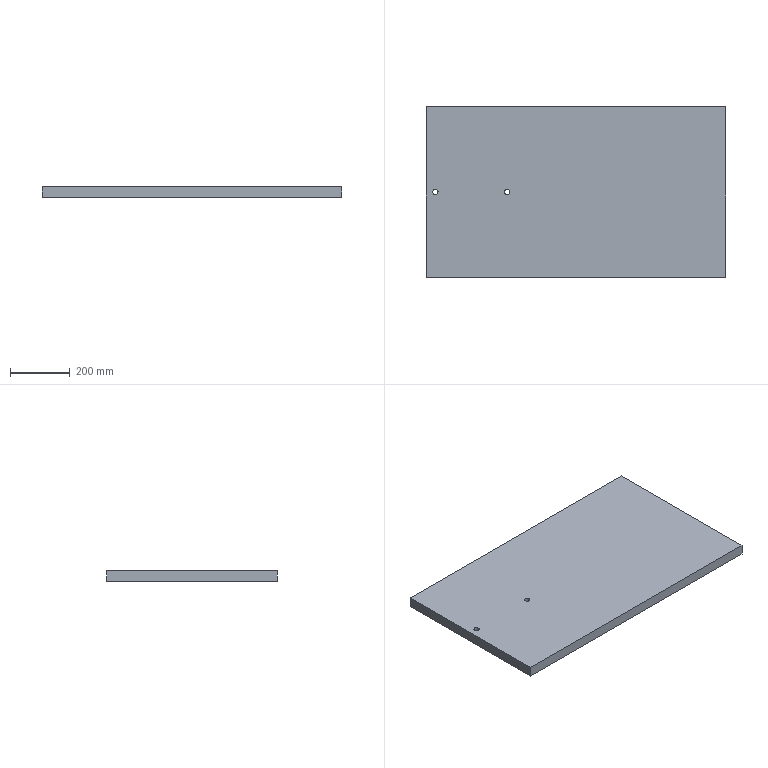Part | SolidWorks | features 3DProfileFeature 1, Extrusion 1, HoleWzd 1 | 1 solid | 10 faces | box 1000 x 570 x 35 mm | volume 19933163 mm3 | plane 6 | cylinder 4 | commonest cylinder face diameters 17.5 x4
STEP:
#1=CARTESIAN_POINT('',(21.25,285.,0.));
#2=VERTEX_POINT('',#1);
#3=CARTESIAN_POINT('',(38.75,285.,0.));
#4=VERTEX_POINT('',#3);
#5=CARTESIAN_POINT('',(30.,285.,0.));
#6=DIRECTION('',(0.,0.,1.));
#7=DIRECTION('',(1.,0.,0.));
#8=AXIS2_PLACEMENT_3D('',#5,#6,#7);
#9=CIRCLE('',#8,8.75);
#10=EDGE_CURVE('',#2,#4,#9,.T.);
#11=ORIENTED_EDGE('',*,*,#10,.F.);
#12=CARTESIAN_POINT('',(21.25,285.,35.));
#13=VERTEX_POINT('',#12);
#14=CARTESIAN_POINT('',(21.25,285.,35.));
#15=DIRECTION('',(0.,0.,1.));
#16=VECTOR('',#15,1000.);
#17=LINE('',#14,#16);
#18=EDGE_CURVE('',#2,#13,#17,.T.);
#19=ORIENTED_EDGE('',*,*,#18,.T.);
#20=CARTESIAN_POINT('',(38.75,285.,35.));
#21=VERTEX_POINT('',#20);
#22=CARTESIAN_POINT('',(30.,285.,35.));
#23=DIRECTION('',(0.,0.,1.));
#24=DIRECTION('',(1.,0.,0.));
#25=AXIS2_PLACEMENT_3D('',#22,#23,#24);
#26=CIRCLE('',#25,8.75);
#27=EDGE_CURVE('',#13,#21,#26,.T.);
#28=ORIENTED_EDGE('',*,*,#27,.T.);
#29=CARTESIAN_POINT('',(38.75,285.,35.));
#30=DIRECTION('',(0.,0.,1.));
#31=VECTOR('',#30,1000.);
#32=LINE('',#29,#31);
#33=EDGE_CURVE('',#4,#21,#32,.T.);
#34=ORIENTED_EDGE('',*,*,#33,.F.);
#35=EDGE_LOOP('',(#11,#19,#28,#34));
#36=FACE_OUTER_BOUND('',#35,.T.);
#37=CARTESIAN_POINT('',(30.,285.,35.));
#38=DIRECTION('',(0.,0.,1.));
#39=DIRECTION('',(1.,0.,0.));
#40=AXIS2_PLACEMENT_3D('',#37,#38,#39);
#41=CYLINDRICAL_SURFACE('',#40,8.75);
#42=ADVANCED_FACE('',(#36),#41,.F.);
#43=CARTESIAN_POINT('',(261.25,285.,0.));
#44=VERTEX_POINT('',#43);
#45=CARTESIAN_POINT('',(278.75,285.,0.));
#46=VERTEX_POINT('',#45);
#47=CARTESIAN_POINT('',(270.,285.,0.));
#48=DIRECTION('',(0.,0.,1.));
#49=DIRECTION('',(1.,0.,0.));
#50=AXIS2_PLACEMENT_3D('',#47,#48,#49);
#51=CIRCLE('',#50,8.75);
#52=EDGE_CURVE('',#44,#46,#51,.T.);
#53=ORIENTED_EDGE('',*,*,#52,.F.);
#54=CARTESIAN_POINT('',(261.25,285.,35.));
#55=VERTEX_POINT('',#54);
#56=CARTESIAN_POINT('',(261.25,285.,35.));
#57=DIRECTION('',(0.,0.,1.));
#58=VECTOR('',#57,1000.);
#59=LINE('',#56,#58);
#60=EDGE_CURVE('',#44,#55,#59,.T.);
#61=ORIENTED_EDGE('',*,*,#60,.T.);
#62=CARTESIAN_POINT('',(278.75,285.,35.));
#63=VERTEX_POINT('',#62);
#64=CARTESIAN_POINT('',(270.,285.,35.));
#65=DIRECTION('',(0.,0.,1.));
#66=DIRECTION('',(1.,0.,0.));
#67=AXIS2_PLACEMENT_3D('',#64,#65,#66);
#68=CIRCLE('',#67,8.75);
#69=EDGE_CURVE('',#55,#63,#68,.T.);
#70=ORIENTED_EDGE('',*,*,#69,.T.);
#71=CARTESIAN_POINT('',(278.75,285.,35.));
#72=DIRECTION('',(0.,0.,1.));
#73=VECTOR('',#72,1000.);
#74=LINE('',#71,#73);
#75=EDGE_CURVE('',#46,#63,#74,.T.);
#76=ORIENTED_EDGE('',*,*,#75,.F.);
#77=EDGE_LOOP('',(#53,#61,#70,#76));
#78=FACE_OUTER_BOUND('',#77,.T.);
#79=CARTESIAN_POINT('',(270.,285.,35.));
#80=DIRECTION('',(0.,0.,1.));
#81=DIRECTION('',(1.,0.,0.));
#82=AXIS2_PLACEMENT_3D('',#79,#80,#81);
#83=CYLINDRICAL_SURFACE('',#82,8.75);
#84=ADVANCED_FACE('',(#78),#83,.F.);
#85=CARTESIAN_POINT('',(0.,0.,0.));
#86=VERTEX_POINT('',#85);
#87=CARTESIAN_POINT('',(1000.,0.,0.));
#88=VERTEX_POINT('',#87);
#89=CARTESIAN_POINT('',(0.,0.,0.));
#90=DIRECTION('',(1.,0.,0.));
#91=VECTOR('',#90,1000.);
#92=LINE('',#89,#91);
#93=EDGE_CURVE('',#86,#88,#92,.T.);
#94=ORIENTED_EDGE('',*,*,#93,.T.);
#95=CARTESIAN_POINT('',(1000.,0.,35.));
#96=VERTEX_POINT('',#95);
#97=CARTESIAN_POINT('',(1000.,0.,35.));
#98=DIRECTION('',(0.,0.,-1.));
#99=VECTOR('',#98,1000.);
#100=LINE('',#97,#99);
#101=EDGE_CURVE('',#96,#88,#100,.T.);
#102=ORIENTED_EDGE('',*,*,#101,.F.);
#103=CARTESIAN_POINT('',(0.,0.,35.));
#104=VERTEX_POINT('',#103);
#105=CARTESIAN_POINT('',(0.,0.,35.));
#106=DIRECTION('',(1.,0.,0.));
#107=VECTOR('',#106,1000.);
#108=LINE('',#105,#107);
#109=EDGE_CURVE('',#104,#96,#108,.T.);
#110=ORIENTED_EDGE('',*,*,#109,.F.);
#111=CARTESIAN_POINT('',(0.,0.,35.));
#112=DIRECTION('',(0.,0.,-1.));
#113=VECTOR('',#112,1000.);
#114=LINE('',#111,#113);
#115=EDGE_CURVE('',#104,#86,#114,.T.);
#116=ORIENTED_EDGE('',*,*,#115,.T.);
#117=EDGE_LOOP('',(#94,#102,#110,#116));
#118=FACE_OUTER_BOUND('',#117,.T.);
#119=CARTESIAN_POINT('',(0.,0.,35.));
#120=DIRECTION('',(0.,1.,0.));
#121=DIRECTION('',(0.,0.,1.));
#122=AXIS2_PLACEMENT_3D('',#119,#120,#121);
#123=PLANE('',#122);
#124=ADVANCED_FACE('',(#118),#123,.F.);
#125=CARTESIAN_POINT('',(1000.,570.,0.));
#126=VERTEX_POINT('',#125);
#127=CARTESIAN_POINT('',(1000.,0.,0.));
#128=DIRECTION('',(0.,1.,0.));
#129=VECTOR('',#128,1000.);
#130=LINE('',#127,#129);
#131=EDGE_CURVE('',#88,#126,#130,.T.);
#132=ORIENTED_EDGE('',*,*,#131,.T.);
#133=CARTESIAN_POINT('',(1000.,570.,35.));
#134=VERTEX_POINT('',#133);
#135=CARTESIAN_POINT('',(1000.,570.,35.));
#136=DIRECTION('',(0.,0.,-1.));
#137=VECTOR('',#136,1000.);
#138=LINE('',#135,#137);
#139=EDGE_CURVE('',#134,#126,#138,.T.);
#140=ORIENTED_EDGE('',*,*,#139,.F.);
#141=CARTESIAN_POINT('',(1000.,0.,35.));
#142=DIRECTION('',(0.,1.,0.));
#143=VECTOR('',#142,1000.);
#144=LINE('',#141,#143);
#145=EDGE_CURVE('',#96,#134,#144,.T.);
#146=ORIENTED_EDGE('',*,*,#145,.F.);
#147=ORIENTED_EDGE('',*,*,#101,.T.);
#148=EDGE_LOOP('',(#132,#140,#146,#147));
#149=FACE_OUTER_BOUND('',#148,.T.);
#150=CARTESIAN_POINT('',(1000.,0.,35.));
#151=DIRECTION('',(-1.,0.,0.));
#152=DIRECTION('',(0.,0.,1.));
#153=AXIS2_PLACEMENT_3D('',#150,#151,#152);
#154=PLANE('',#153);
#155=ADVANCED_FACE('',(#149),#154,.F.);
#156=CARTESIAN_POINT('',(0.,570.,0.));
#157=VERTEX_POINT('',#156);
#158=CARTESIAN_POINT('',(0.,570.,0.));
#159=DIRECTION('',(-1.,0.,0.));
#160=VECTOR('',#159,1000.);
#161=LINE('',#158,#160);
#162=EDGE_CURVE('',#126,#157,#161,.T.);
#163=ORIENTED_EDGE('',*,*,#162,.T.);
#164=CARTESIAN_POINT('',(0.,570.,35.));
#165=VERTEX_POINT('',#164);
#166=CARTESIAN_POINT('',(0.,570.,35.));
#167=DIRECTION('',(0.,0.,-1.));
#168=VECTOR('',#167,1000.);
#169=LINE('',#166,#168);
#170=EDGE_CURVE('',#165,#157,#169,.T.);
#171=ORIENTED_EDGE('',*,*,#170,.F.);
#172=CARTESIAN_POINT('',(0.,570.,35.));
#173=DIRECTION('',(-1.,0.,0.));
#174=VECTOR('',#173,1000.);
#175=LINE('',#172,#174);
#176=EDGE_CURVE('',#134,#165,#175,.T.);
#177=ORIENTED_EDGE('',*,*,#176,.F.);
#178=ORIENTED_EDGE('',*,*,#139,.T.);
#179=EDGE_LOOP('',(#163,#171,#177,#178));
#180=FACE_OUTER_BOUND('',#179,.T.);
#181=CARTESIAN_POINT('',(0.,570.,35.));
#182=DIRECTION('',(0.,-1.,0.));
#183=DIRECTION('',(0.,0.,-1.));
#184=AXIS2_PLACEMENT_3D('',#181,#182,#183);
#185=PLANE('',#184);
#186=ADVANCED_FACE('',(#180),#185,.F.);
#187=CARTESIAN_POINT('',(0.,0.,0.));
#188=DIRECTION('',(0.,-1.,0.));
#189=VECTOR('',#188,1000.);
#190=LINE('',#187,#189);
#191=EDGE_CURVE('',#157,#86,#190,.T.);
#192=ORIENTED_EDGE('',*,*,#191,.T.);
#193=ORIENTED_EDGE('',*,*,#115,.F.);
#194=CARTESIAN_POINT('',(0.,0.,35.));
#195=DIRECTION('',(0.,-1.,0.));
#196=VECTOR('',#195,1000.);
#197=LINE('',#194,#196);
#198=EDGE_CURVE('',#165,#104,#197,.T.);
#199=ORIENTED_EDGE('',*,*,#198,.F.);
#200=ORIENTED_EDGE('',*,*,#170,.T.);
#201=EDGE_LOOP('',(#192,#193,#199,#200));
#202=FACE_OUTER_BOUND('',#201,.T.);
#203=CARTESIAN_POINT('',(0.,0.,35.));
#204=DIRECTION('',(1.,0.,0.));
#205=DIRECTION('',(0.,0.,-1.));
#206=AXIS2_PLACEMENT_3D('',#203,#204,#205);
#207=PLANE('',#206);
#208=ADVANCED_FACE('',(#202),#207,.F.);
#209=CARTESIAN_POINT('',(30.,285.,35.));
#210=DIRECTION('',(0.,0.,1.));
#211=DIRECTION('',(1.,0.,0.));
#212=AXIS2_PLACEMENT_3D('',#209,#210,#211);
#213=CIRCLE('',#212,8.75);
#214=EDGE_CURVE('',#21,#13,#213,.T.);
#215=ORIENTED_EDGE('',*,*,#214,.F.);
#216=ORIENTED_EDGE('',*,*,#27,.F.);
#217=EDGE_LOOP('',(#215,#216));
#218=FACE_BOUND('',#217,.T.);
#219=CARTESIAN_POINT('',(270.,285.,35.));
#220=DIRECTION('',(0.,0.,1.));
#221=DIRECTION('',(1.,0.,0.));
#222=AXIS2_PLACEMENT_3D('',#219,#220,#221);
#223=CIRCLE('',#222,8.75);
#224=EDGE_CURVE('',#63,#55,#223,.T.);
#225=ORIENTED_EDGE('',*,*,#224,.F.);
#226=ORIENTED_EDGE('',*,*,#69,.F.);
#227=EDGE_LOOP('',(#225,#226));
#228=FACE_BOUND('',#227,.T.);
#229=ORIENTED_EDGE('',*,*,#109,.T.);
#230=ORIENTED_EDGE('',*,*,#145,.T.);
#231=ORIENTED_EDGE('',*,*,#176,.T.);
#232=ORIENTED_EDGE('',*,*,#198,.T.);
#233=EDGE_LOOP('',(#229,#230,#231,#232));
#234=FACE_OUTER_BOUND('',#233,.T.);
#235=CARTESIAN_POINT('',(0.,0.,35.));
#236=DIRECTION('',(0.,0.,1.));
#237=DIRECTION('',(1.,0.,0.));
#238=AXIS2_PLACEMENT_3D('',#235,#236,#237);
#239=PLANE('',#238);
#240=ADVANCED_FACE('',(#218,#228,#234),#239,.T.);
#241=CARTESIAN_POINT('',(30.,285.,0.));
#242=DIRECTION('',(0.,0.,1.));
#243=DIRECTION('',(1.,0.,0.));
#244=AXIS2_PLACEMENT_3D('',#241,#242,#243);
#245=CIRCLE('',#244,8.75);
#246=EDGE_CURVE('',#4,#2,#245,.T.);
#247=ORIENTED_EDGE('',*,*,#246,.T.);
#248=ORIENTED_EDGE('',*,*,#10,.T.);
#249=EDGE_LOOP('',(#247,#248));
#250=FACE_BOUND('',#249,.T.);
#251=CARTESIAN_POINT('',(270.,285.,0.));
#252=DIRECTION('',(0.,0.,1.));
#253=DIRECTION('',(1.,0.,0.));
#254=AXIS2_PLACEMENT_3D('',#251,#252,#253);
#255=CIRCLE('',#254,8.75);
#256=EDGE_CURVE('',#46,#44,#255,.T.);
#257=ORIENTED_EDGE('',*,*,#256,.T.);
#258=ORIENTED_EDGE('',*,*,#52,.T.);
#259=EDGE_LOOP('',(#257,#258));
#260=FACE_BOUND('',#259,.T.);
#261=ORIENTED_EDGE('',*,*,#93,.F.);
#262=ORIENTED_EDGE('',*,*,#191,.F.);
#263=ORIENTED_EDGE('',*,*,#162,.F.);
#264=ORIENTED_EDGE('',*,*,#131,.F.);
#265=EDGE_LOOP('',(#261,#262,#263,#264));
#266=FACE_OUTER_BOUND('',#265,.T.);
#267=CARTESIAN_POINT('',(0.,0.,0.));
#268=DIRECTION('',(0.,0.,1.));
#269=DIRECTION('',(1.,0.,0.));
#270=AXIS2_PLACEMENT_3D('',#267,#268,#269);
#271=PLANE('',#270);
#272=ADVANCED_FACE('',(#250,#260,#266),#271,.F.);
#273=ORIENTED_EDGE('',*,*,#60,.F.);
#274=ORIENTED_EDGE('',*,*,#256,.F.);
#275=ORIENTED_EDGE('',*,*,#75,.T.);
#276=ORIENTED_EDGE('',*,*,#224,.T.);
#277=EDGE_LOOP('',(#273,#274,#275,#276));
#278=FACE_OUTER_BOUND('',#277,.T.);
#279=CARTESIAN_POINT('',(270.,285.,35.));
#280=DIRECTION('',(0.,0.,1.));
#281=DIRECTION('',(1.,0.,0.));
#282=AXIS2_PLACEMENT_3D('',#279,#280,#281);
#283=CYLINDRICAL_SURFACE('',#282,8.75);
#284=ADVANCED_FACE('',(#278),#283,.F.);
#285=ORIENTED_EDGE('',*,*,#18,.F.);
#286=ORIENTED_EDGE('',*,*,#246,.F.);
#287=ORIENTED_EDGE('',*,*,#33,.T.);
#288=ORIENTED_EDGE('',*,*,#214,.T.);
#289=EDGE_LOOP('',(#285,#286,#287,#288));
#290=FACE_OUTER_BOUND('',#289,.T.);
#291=CARTESIAN_POINT('',(30.,285.,35.));
#292=DIRECTION('',(0.,0.,1.));
#293=DIRECTION('',(1.,0.,0.));
#294=AXIS2_PLACEMENT_3D('',#291,#292,#293);
#295=CYLINDRICAL_SURFACE('',#294,8.75);
#296=ADVANCED_FACE('',(#290),#295,.F.);
#297=CLOSED_SHELL('',(#42,#84,#124,#155,#186,#208,#240,#272,#284,#296));
#298=MANIFOLD_SOLID_BREP('',#297);
#299=CARTESIAN_POINT('',(0.,0.,0.));
#300=DIRECTION('',(0.,0.,1.));
#301=DIRECTION('',(1.,0.,0.));
#302=AXIS2_PLACEMENT_3D('',#299,#300,#301);
#303=(LENGTH_UNIT()NAMED_UNIT(*)SI_UNIT(.MILLI.,.METRE.));
#304=UNCERTAINTY_MEASURE_WITH_UNIT(LENGTH_MEASURE(0.00001),#303,'','');
#305=(NAMED_UNIT(*)PLANE_ANGLE_UNIT()SI_UNIT($,.RADIAN.));
#306=(NAMED_UNIT(*)SI_UNIT($,.STERADIAN.)SOLID_ANGLE_UNIT());
#307=(GEOMETRIC_REPRESENTATION_CONTEXT(3)GLOBAL_UNCERTAINTY_ASSIGNED_CONTEXT((#304))GLOBAL_UNIT_ASSIGNED_CONTEXT((#303,#305,#306))REPRESENTATION_CONTEXT('',''));
#308=ADVANCED_BREP_SHAPE_REPRESENTATION('',(#298,#302),#307);